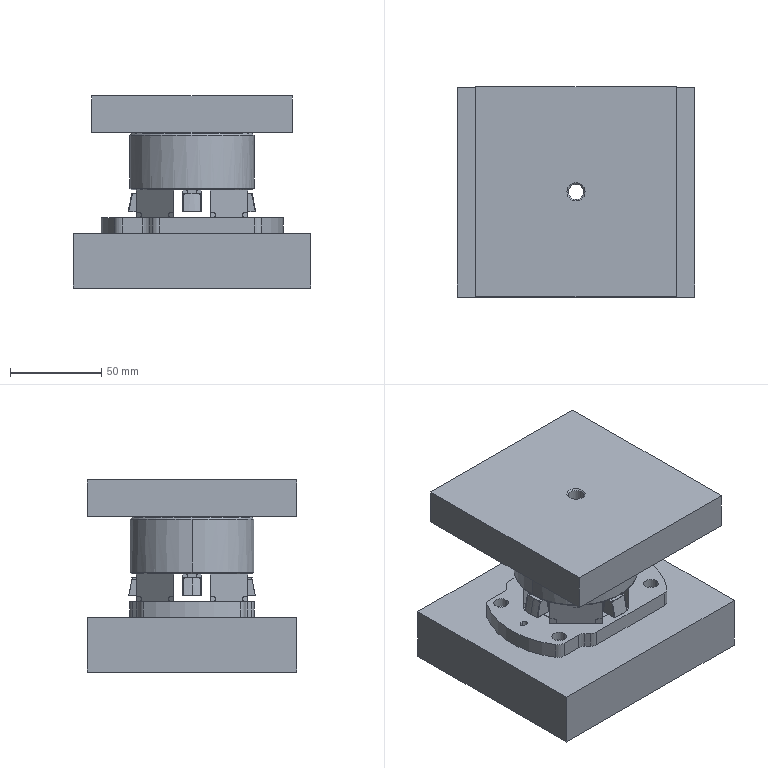NC program | NX | posted with a generic post | part box 130 x 115 x 105.2 mm
Lines 1 to 950 of 2949:
N10 G17 G21 G94 G90
(PLANAR_MILL_COPY_4_COPY_3_COPY_1 , TOOL : D2)
N12 T20 M6
N14 G54
N16 G17 G0 G90 X-1.137 Y30.713 S6000 M3
N18 G43 Z52.144 H20
N20 G94 G1 Y9.394 Z30.825 F5000.
N22 G41 X-1. Y9.659 Z30.559 F1200. D20
N24 Y11.721 Z28.498
N26 X-1.018 Y11.795 Z28.423
N28 X-1.095 Y11.849 Z28.369
N30 X-1.2 Y11.862 Z28.356
N32 X-1.8
N34 X-1.905 Y11.849 Z28.369
N36 X-1.982 Y11.795 Z28.423
N38 X-2. Y11.721 Z28.498
N40 Y9.894 Z30.324
N42 X-1.966 Y9.827 Z30.391
N44 G40
N46 X-1.863 Y9.628 Z30.59
N48 G0 X-1.137 Y9.288 Z30.719
N50 G41 G1 X-1. Y9.553 Z30.453
N52 Y11.615 Z28.392
N54 X-1.018 Y11.689 Z28.317
N56 X-1.095 Y11.743 Z28.263
N58 X-1.2 Y11.756 Z28.25
N60 X-1.8
N62 X-1.905 Y11.743 Z28.263
N64 X-1.982 Y11.689 Z28.317
N66 X-2. Y11.615 Z28.392
N68 Y9.788 Z30.218
N70 X-1.966 Y9.721 Z30.285
N72 G40
N74 X-1.863 Y9.522 Z30.484
N76 G0 X-1.137 Y9.182 Z30.613
N78 G41 G1 X-1. Y9.447 Z30.347
N80 Y11.509 Z28.286
N82 X-1.018 Y11.583 Z28.211
N84 X-1.095 Y11.637 Z28.157
N86 X-1.2 Y11.65 Z28.144
N88 X-1.8
N90 X-1.905 Y11.637 Z28.157
N92 X-1.982 Y11.583 Z28.211
N94 X-2. Y11.509 Z28.286
N96 Y9.682 Z30.112
N98 X-1.966 Y9.615 Z30.179
N100 G40
N102 X-1.863 Y9.416 Z30.378
N104 G0 X-1.137 Y9.076 Z30.507
N106 G41 G1 X-1. Y9.341 Z30.241
N108 Y11.403 Z28.179
N110 X-1.018 Y11.477 Z28.105
N112 X-1.095 Y11.531 Z28.051
N114 X-1.2 Y11.544 Z28.038
N116 X-1.8
N118 X-1.905 Y11.531 Z28.051
N120 X-1.982 Y11.477 Z28.105
N122 X-2. Y11.403 Z28.179
N124 Y9.576 Z30.006
N126 X-1.966 Y9.509 Z30.073
N128 G40
N130 X-1.863 Y9.31 Z30.272
N132 G0 X-1.137 Y8.969 Z30.4
N134 G41 G1 X-1. Y9.235 Z30.135
N136 Y11.296 Z28.073
N138 X-1.018 Y11.371 Z27.999
N140 X-1.095 Y11.425 Z27.945
N142 X-1.2 Y11.438 Z27.932
N144 X-1.8
N146 X-1.905 Y11.425 Z27.945
N148 X-1.982 Y11.371 Z27.999
N150 X-2. Y11.296 Z28.073
N152 Y9.47 Z29.9
N154 X-1.966 Y9.403 Z29.967
N156 G40
N158 X-1.863 Y9.204 Z30.166
N160 G0 X-1.137 Y8.863 Z30.294
N162 G41 G1 X-1. Y9.129 Z30.029
N164 Y11.19 Z27.967
N166 X-1.018 Y11.265 Z27.893
N168 X-1.095 Y11.319 Z27.839
N170 X-1.2 Y11.332 Z27.826
N172 X-1.8
N174 X-1.905 Y11.319 Z27.839
N176 X-1.982 Y11.265 Z27.893
N178 X-2. Y11.19 Z27.967
N180 Y9.364 Z29.794
N182 X-1.966 Y9.297 Z29.861
N184 G40
N186 X-1.863 Y9.098 Z30.06
N188 G0 X-1.137 Y8.757 Z30.188
N190 G41 G1 X-1. Y9.023 Z29.923
N192 Y11.084 Z27.861
N194 X-1.018 Y11.159 Z27.787
N196 X-1.095 Y11.213 Z27.733
N198 X-1.2 Y11.226 Z27.72
N200 X-1.8
N202 X-1.905 Y11.213 Z27.733
N204 X-1.982 Y11.159 Z27.787
N206 X-2. Y11.084 Z27.861
N208 Y9.258 Z29.688
N210 X-1.966 Y9.191 Z29.755
N212 G40
N214 X-1.863 Y8.992 Z29.954
N216 G0 X-1.137 Y8.651 Z30.082
N218 G41 G1 X-1. Y8.917 Z29.816
N220 Y10.978 Z27.755
N222 X-1.018 Y11.053 Z27.681
N224 X-1.095 Y11.107 Z27.627
N226 X-1.2 Y11.12 Z27.614
N228 X-1.8
N230 X-1.905 Y11.107 Z27.627
N232 X-1.982 Y11.053 Z27.681
N234 X-2. Y10.978 Z27.755
N236 Y9.151 Z29.582
N238 X-1.966 Y9.085 Z29.648
N240 G40
N242 X-1.863 Y8.886 Z29.848
N244 G0 X-1.137 Y8.545 Z29.976
N246 G41 G1 X-1. Y8.811 Z29.71
N248 Y10.872 Z27.649
N250 X-1.018 Y10.946 Z27.575
N252 X-1.095 Y11.001 Z27.521
N254 X-1.2 Y11.014 Z27.508
N256 X-1.8
N258 X-1.905 Y11.001 Z27.521
N260 X-1.982 Y10.946 Z27.575
N262 X-2. Y10.872 Z27.649
N264 Y9.045 Z29.476
N266 X-1.966 Y8.979 Z29.542
N268 G40
N270 X-1.863 Y8.78 Z29.742
N272 G0 X-1.137 Y8.439 Z29.87
N274 G41 G1 X-1. Y8.705 Z29.604
N276 Y10.766 Z27.543
N278 X-1.018 Y10.84 Z27.469
N280 X-1.095 Y10.895 Z27.414
N282 X-1.2 Y10.908 Z27.402
N284 X-1.8
N286 X-1.905 Y10.895 Z27.414
N288 X-1.982 Y10.84 Z27.469
N290 X-2. Y10.766 Z27.543
N292 Y8.939 Z29.37
N294 X-1.966 Y8.873 Z29.436
N296 G40
N298 X-1.863 Y8.674 Z29.636
N300 G0 X-1.137 Y8.333 Z29.764
N302 G41 G1 X-1. Y8.599 Z29.498
N304 Y10.66 Z27.437
N306 X-1.018 Y10.734 Z27.363
N308 X-1.095 Y10.789 Z27.308
N310 X-1.2 Y10.802 Z27.296
N312 X-1.8
N314 X-1.905 Y10.789 Z27.308
N316 X-1.982 Y10.734 Z27.363
N318 X-2. Y10.66 Z27.437
N320 Y8.833 Z29.264
N322 X-1.966 Y8.767 Z29.33
N324 G40
N326 X-1.863 Y8.567 Z29.53
N328 G0 X-1.137 Y8.227 Z29.658
N330 G41 G1 X-1. Y8.493 Z29.392
N332 Y10.554 Z27.331
N334 X-1.018 Y10.628 Z27.257
N336 X-1.095 Y10.683 Z27.202
N338 X-1.2 Y10.695 Z27.19
N340 X-1.8
N342 X-1.905 Y10.683 Z27.202
N344 X-1.982 Y10.628 Z27.257
N346 X-2. Y10.554 Z27.331
N348 Y8.727 Z29.158
N350 X-1.966 Y8.661 Z29.224
N352 G40
N354 X-1.863 Y8.461 Z29.424
N356 G0 X-1.137 Y8.121 Z29.552
N358 G41 G1 X-1. Y8.387 Z29.286
N360 Y10.448 Z27.225
N362 X-1.018 Y10.522 Z27.151
N364 X-1.095 Y10.577 Z27.096
N366 X-1.2 Y10.589 Z27.083
N368 X-1.8
N370 X-1.905 Y10.577 Z27.096
N372 X-1.982 Y10.522 Z27.151
N374 X-2. Y10.448 Z27.225
N376 Y8.621 Z29.052
N378 X-1.966 Y8.555 Z29.118
N380 G40
N382 X-1.863 Y8.355 Z29.317
N384 G0 X-1.137 Y8.015 Z29.446
N386 G41 G1 X-1. Y8.281 Z29.18
N388 Y10.342 Z27.119
N390 X-1.018 Y10.416 Z27.045
N392 X-1.095 Y10.47 Z26.99
N394 X-1.2 Y10.483 Z26.977
N396 X-1.8
N398 X-1.905 Y10.47 Z26.99
N400 X-1.982 Y10.416 Z27.045
N402 X-2. Y10.342 Z27.119
N404 Y8.515 Z28.946
N406 X-1.966 Y8.449 Z29.012
N408 G40
N410 X-1.863 Y8.249 Z29.211
N412 G0 X-1.137 Y7.909 Z29.34
N414 G41 G1 X-1. Y8.175 Z29.074
N416 Y10.236 Z27.013
N418 X-1.018 Y10.31 Z26.939
N420 X-1.095 Y10.364 Z26.884
N422 X-1.2 Y10.377 Z26.871
N424 X-1.8
N426 X-1.905 Y10.364 Z26.884
N428 X-1.982 Y10.31 Z26.939
N430 X-2. Y10.236 Z27.013
N432 Y8.409 Z28.84
N434 X-1.966 Y8.343 Z28.906
N436 G40
N438 X-1.863 Y8.143 Z29.105
N440 G0 X-1.137 Y7.803 Z29.234
N442 G41 G1 X-1. Y8.069 Z28.968
N444 Y10.13 Z26.907
N446 X-1.018 Y10.204 Z26.832
N448 X-1.095 Y10.258 Z26.778
N450 X-1.2 Y10.271 Z26.765
N452 X-1.8
N454 X-1.905 Y10.258 Z26.778
N456 X-1.982 Y10.204 Z26.832
N458 X-2. Y10.13 Z26.907
N460 Y8.303 Z28.734
N462 X-1.966 Y8.236 Z28.8
N464 G40
N466 X-1.863 Y8.037 Z28.999
N468 G0 X-1.137 Y7.697 Z29.128
N470 G41 G1 X-1. Y7.962 Z28.862
N472 Y10.024 Z26.801
N474 X-1.018 Y10.098 Z26.726
N476 X-1.095 Y10.152 Z26.672
N478 X-1.2 Y10.165 Z26.659
N480 X-1.8
N482 X-1.905 Y10.152 Z26.672
N484 X-1.982 Y10.098 Z26.726
N486 X-2. Y10.024 Z26.801
N488 Y8.197 Z28.627
N490 X-1.966 Y8.13 Z28.694
N492 G40
N494 X-1.863 Y7.931 Z28.893
N496 G0 X-1.137 Y7.591 Z29.022
N498 G41 G1 X-1. Y7.856 Z28.756
N500 Y9.918 Z26.695
N502 X-1.018 Y9.992 Z26.62
N504 X-1.095 Y10.046 Z26.566
N506 X-1.2 Y10.059 Z26.553
N508 X-1.8
N510 X-1.905 Y10.046 Z26.566
N512 X-1.982 Y9.992 Z26.62
N514 X-2. Y9.918 Z26.695
N516 Y8.091 Z28.521
N518 X-1.966 Y8.024 Z28.588
N520 G40
N522 X-1.863 Y7.825 Z28.787
N524 G0 X-1.137 Y7.485 Z28.916
N526 G41 G1 X-1. Y7.75 Z28.65
N528 Y9.812 Z26.588
N530 X-1.018 Y9.886 Z26.514
N532 X-1.095 Y9.94 Z26.46
N534 X-1.2 Y9.953 Z26.447
N536 X-1.8
N538 X-1.905 Y9.94 Z26.46
N540 X-1.982 Y9.886 Z26.514
N542 X-2. Y9.812 Z26.588
N544 Y7.985 Z28.415
N546 X-1.966 Y7.918 Z28.482
N548 G40
N550 X-1.863 Y7.719 Z28.681
N552 G0 X-1.137 Y7.378 Z28.809
N554 G41 G1 X-1. Y7.644 Z28.544
N556 Y9.705 Z26.482
N558 X-1.018 Y9.78 Z26.408
N560 X-1.095 Y9.834 Z26.354
N562 X-1.2 Y9.847 Z26.341
N564 X-1.8
N566 X-1.905 Y9.834 Z26.354
N568 X-1.982 Y9.78 Z26.408
N570 X-2. Y9.705 Z26.482
N572 Y7.879 Z28.309
N574 X-1.966 Y7.812 Z28.376
N576 G40
N578 X-1.863 Y7.613 Z28.575
N580 G0 X-1.137 Y7.272 Z28.703
N582 G41 G1 X-1. Y7.538 Z28.438
N584 Y9.599 Z26.376
N586 X-1.018 Y9.674 Z26.302
N588 X-1.095 Y9.728 Z26.248
N590 X-1.2 Y9.741 Z26.235
N592 X-1.8
N594 X-1.905 Y9.728 Z26.248
N596 X-1.982 Y9.674 Z26.302
N598 X-2. Y9.599 Z26.376
N600 Y7.773 Z28.203
N602 X-1.966 Y7.706 Z28.27
N604 G40
N606 X-1.863 Y7.507 Z28.469
N608 G0 X-1.137 Y7.166 Z28.597
N610 G41 G1 X-1. Y7.432 Z28.332
N612 Y9.493 Z26.27
N614 X-1.018 Y9.568 Z26.196
N616 X-1.095 Y9.622 Z26.142
N618 X-1.2 Y9.635 Z26.129
N620 X-1.8
N622 X-1.905 Y9.622 Z26.142
N624 X-1.982 Y9.568 Z26.196
N626 X-2. Y9.493 Z26.27
N628 Y7.667 Z28.097
N630 X-1.966 Y7.6 Z28.164
N632 G40
N634 X-1.863 Y7.401 Z28.363
N636 G0 X-1.137 Y7.06 Z28.491
N638 G41 G1 X-1. Y7.326 Z28.225
N640 Y9.387 Z26.164
N642 X-1.018 Y9.462 Z26.09
N644 X-1.095 Y9.516 Z26.036
N646 X-1.2 Y9.529 Z26.023
N648 X-1.8
N650 X-1.905 Y9.516 Z26.036
N652 X-1.982 Y9.462 Z26.09
N654 X-2. Y9.387 Z26.164
N656 Y7.56 Z27.991
N658 X-1.966 Y7.494 Z28.057
N660 G40
N662 X-1.863 Y7.295 Z28.257
N664 G0 X-1.137 Y6.954 Z28.385
N666 G41 G1 X-1. Y7.22 Z28.119
N668 Y9.281 Z26.058
N670 X-1.018 Y9.355 Z25.984
N672 X-1.095 Y9.41 Z25.93
N674 X-1.2 Y9.423 Z25.917
N676 X-1.8
N678 X-1.905 Y9.41 Z25.93
N680 X-1.982 Y9.355 Z25.984
N682 X-2. Y9.281 Z26.058
N684 Y7.454 Z27.885
N686 X-1.966 Y7.388 Z27.951
N688 G40
N690 X-1.863 Y7.189 Z28.151
N692 G0 X-1.137 Y6.848 Z28.279
N694 G41 G1 X-1. Y7.114 Z28.013
N696 Y9.175 Z25.952
N698 X-1.018 Y9.249 Z25.878
N700 X-1.095 Y9.304 Z25.824
N702 X-1.2 Y9.317 Z25.811
N704 X-1.8
N706 X-1.905 Y9.304 Z25.824
N708 X-1.982 Y9.249 Z25.878
N710 X-2. Y9.175 Z25.952
N712 Y7.348 Z27.779
N714 X-1.966 Y7.282 Z27.845
N716 G40
N718 X-1.863 Y7.083 Z28.045
N720 G0 X-1.137 Y6.813 Z28.244
N722 G41 G1 X-1. Y7.079 Z27.978
N724 Y9.14 Z25.917
N726 X-1.018 Y9.214 Z25.843
N728 X-1.095 Y9.268 Z25.788
N730 X-1.2 Y9.281 Z25.775
N732 X-1.8
N734 X-1.905 Y9.268 Z25.788
N736 X-1.982 Y9.214 Z25.843
N738 X-2. Y9.14 Z25.917
N740 Y7.313 Z27.744
N742 X-1.966 Y7.247 Z27.81
N744 G40
N746 X-1.863 Y7.047 Z28.009
N748 G0 Y27.412 Z48.374
N750 Y48.374 Z27.412
N752 G1 Y30.59 Z9.628 F5000.
N754 G41 X-2. Y30.324 Z9.894 F1200.
N756 Y28.498 Z11.721
N758 X-1.982 Y28.423 Z11.795
N760 X-1.905 Y28.369 Z11.849
N762 X-1.8 Y28.356 Z11.862
N764 X-1.2
N766 X-1.095 Y28.369 Z11.849
N768 X-1.018 Y28.423 Z11.795
N770 X-1. Y28.498 Z11.721
N772 Y30.559 Z9.659
N774 X-1.034 Y30.625 Z9.593
N776 G40
N778 X-1.137 Y30.825 Z9.394
N780 G0 X-1.863 Y30.484 Z9.522
N782 G41 G1 X-2. Y30.218 Z9.788
N784 Y28.392 Z11.615
N786 X-1.982 Y28.317 Z11.689
N788 X-1.905 Y28.263 Z11.743
N790 X-1.8 Y28.25 Z11.756
N792 X-1.2
N794 X-1.095 Y28.263 Z11.743
N796 X-1.018 Y28.317 Z11.689
N798 X-1. Y28.392 Z11.615
N800 Y30.453 Z9.553
N802 X-1.034 Y30.519 Z9.487
N804 G40
N806 X-1.137 Y30.719 Z9.288
N808 G0 X-1.863 Y30.378 Z9.416
N810 G41 G1 X-2. Y30.112 Z9.682
N812 Y28.286 Z11.509
N814 X-1.982 Y28.211 Z11.583
N816 X-1.905 Y28.157 Z11.637
N818 X-1.8 Y28.144 Z11.65
N820 X-1.2
N822 X-1.095 Y28.157 Z11.637
N824 X-1.018 Y28.211 Z11.583
N826 X-1. Y28.286 Z11.509
N828 Y30.347 Z9.447
N830 X-1.034 Y30.413 Z9.381
N832 G40
N834 X-1.137 Y30.613 Z9.182
N836 G0 X-1.863 Y30.272 Z9.31
N838 G41 G1 X-2. Y30.006 Z9.576
N840 Y28.179 Z11.403
N842 X-1.982 Y28.105 Z11.477
N844 X-1.905 Y28.051 Z11.531
N846 X-1.8 Y28.038 Z11.544
N848 X-1.2
N850 X-1.095 Y28.051 Z11.531
N852 X-1.018 Y28.105 Z11.477
N854 X-1. Y28.179 Z11.403
N856 Y30.241 Z9.341
N858 X-1.034 Y30.307 Z9.275
N860 G40
N862 X-1.137 Y30.507 Z9.076
N864 G0 X-1.863 Y30.166 Z9.204
N866 G41 G1 X-2. Y29.9 Z9.47
N868 Y28.073 Z11.296
N870 X-1.982 Y27.999 Z11.371
N872 X-1.905 Y27.945 Z11.425
N874 X-1.8 Y27.932 Z11.438
N876 X-1.2
N878 X-1.095 Y27.945 Z11.425
N880 X-1.018 Y27.999 Z11.371
N882 X-1. Y28.073 Z11.296
N884 Y30.135 Z9.235
N886 X-1.034 Y30.201 Z9.169
N888 G40
N890 X-1.137 Y30.4 Z8.969
N892 G0 X-1.863 Y30.06 Z9.098
N894 G41 G1 X-2. Y29.794 Z9.364
N896 Y27.967 Z11.19
N898 X-1.982 Y27.893 Z11.265
N900 X-1.905 Y27.839 Z11.319
N902 X-1.8 Y27.826 Z11.332
N904 X-1.2
N906 X-1.095 Y27.839 Z11.319
N908 X-1.018 Y27.893 Z11.265
N910 X-1. Y27.967 Z11.19
N912 Y30.029 Z9.129
N914 X-1.034 Y30.095 Z9.063
N916 G40
N918 X-1.137 Y30.294 Z8.863
N920 G0 X-1.863 Y29.954 Z8.992
N922 G41 G1 X-2. Y29.688 Z9.258
N924 Y27.861 Z11.084
N926 X-1.982 Y27.787 Z11.159
N928 X-1.905 Y27.733 Z11.213
N930 X-1.8 Y27.72 Z11.226
N932 X-1.2
N934 X-1.095 Y27.733 Z11.213
N936 X-1.018 Y27.787 Z11.159
N938 X-1. Y27.861 Z11.084
N940 Y29.923 Z9.023
N942 X-1.034 Y29.989 Z8.957
N944 G40
N946 X-1.137 Y30.188 Z8.757
N948 G0 X-1.863 Y29.848 Z8.886
N950 G41 G1 X-2. Y29.582 Z9.151
N952 Y27.755 Z10.978
N954 X-1.982 Y27.681 Z11.053
N956 X-1.905 Y27.627 Z11.107
N958 X-1.8 Y27.614 Z11.12
N960 X-1.2
N962 X-1.095 Y27.627 Z11.107
N964 X-1.018 Y27.681 Z11.053
N966 X-1. Y27.755 Z10.978
N968 Y29.816 Z8.917
N970 X-1.034 Y29.883 Z8.851
N972 G40
N974 X-1.137 Y30.082 Z8.651
N976 G0 X-1.863 Y29.742 Z8.78
N978 G41 G1 X-2. Y29.476 Z9.045
N980 Y27.649 Z10.872
N982 X-1.982 Y27.575 Z10.946
N984 X-1.905 Y27.521 Z11.001
N986 X-1.8 Y27.508 Z11.014
N988 X-1.2
N990 X-1.095 Y27.521 Z11.001
N992 X-1.018 Y27.575 Z10.946
N994 X-1. Y27.649 Z10.872
N996 Y29.71 Z8.811
N998 X-1.034 Y29.777 Z8.745
N1000 G40
N1002 X-1.137 Y29.976 Z8.545
N1004 G0 X-1.863 Y29.636 Z8.674
N1006 G41 G1 X-2. Y29.37 Z8.939
N1008 Y27.543 Z10.766
N1010 X-1.982 Y27.469 Z10.84
N1012 X-1.905 Y27.414 Z10.895
N1014 X-1.8 Y27.402 Z10.908
N1016 X-1.2
N1018 X-1.095 Y27.414 Z10.895
N1020 X-1.018 Y27.469 Z10.84
N1022 X-1. Y27.543 Z10.766
N1024 Y29.604 Z8.705
N1026 X-1.034 Y29.671 Z8.638
N1028 G40
N1030 X-1.137 Y29.87 Z8.439
N1032 G0 X-1.863 Y29.53 Z8.567
N1034 G41 G1 X-2. Y29.264 Z8.833
N1036 Y27.437 Z10.66
N1038 X-1.982 Y27.363 Z10.734
N1040 X-1.905 Y27.308 Z10.789
N1042 X-1.8 Y27.296 Z10.802
N1044 X-1.2
N1046 X-1.095 Y27.308 Z10.789
N1048 X-1.018 Y27.363 Z10.734
N1050 X-1. Y27.437 Z10.66
N1052 Y29.498 Z8.599
N1054 X-1.034 Y29.565 Z8.532
N1056 G40
N1058 X-1.137 Y29.764 Z8.333
N1060 G0 X-1.863 Y29.424 Z8.461
N1062 G41 G1 X-2. Y29.158 Z8.727
N1064 Y27.331 Z10.554
N1066 X-1.982 Y27.257 Z10.628
N1068 X-1.905 Y27.202 Z10.683
N1070 X-1.8 Y27.19 Z10.695
N1072 X-1.2
N1074 X-1.095 Y27.202 Z10.683
N1076 X-1.018 Y27.257 Z10.628
N1078 X-1. Y27.331 Z10.554
N1080 Y29.392 Z8.493
N1082 X-1.034 Y29.459 Z8.426
N1084 G40
N1086 X-1.137 Y29.658 Z8.227
N1088 G0 X-1.863 Y29.317 Z8.355
N1090 G41 G1 X-2. Y29.052 Z8.621
N1092 Y27.225 Z10.448
N1094 X-1.982 Y27.151 Z10.522
N1096 X-1.905 Y27.096 Z10.577
N1098 X-1.8 Y27.083 Z10.589
N1100 X-1.2
N1102 X-1.095 Y27.096 Z10.577
N1104 X-1.018 Y27.151 Z10.522
N1106 X-1. Y27.225 Z10.448
N1108 Y29.286 Z8.387
N1110 X-1.034 Y29.353 Z8.32
N1112 G40
N1114 X-1.137 Y29.552 Z8.121
N1116 G0 X-1.863 Y29.211 Z8.249
N1118 G41 G1 X-2. Y28.946 Z8.515
N1120 Y27.119 Z10.342
N1122 X-1.982 Y27.045 Z10.416
N1124 X-1.905 Y26.99 Z10.47
N1126 X-1.8 Y26.977 Z10.483
N1128 X-1.2
N1130 X-1.095 Y26.99 Z10.47
N1132 X-1.018 Y27.045 Z10.416
N1134 X-1. Y27.119 Z10.342
N1136 Y29.18 Z8.281
N1138 X-1.034 Y29.247 Z8.214
N1140 G40
N1142 X-1.137 Y29.446 Z8.015
N1144 G0 X-1.863 Y29.105 Z8.143
N1146 G41 G1 X-2. Y28.84 Z8.409
N1148 Y27.013 Z10.236
N1150 X-1.982 Y26.939 Z10.31
N1152 X-1.905 Y26.884 Z10.364
N1154 X-1.8 Y26.871 Z10.377
N1156 X-1.2
N1158 X-1.095 Y26.884 Z10.364
N1160 X-1.018 Y26.939 Z10.31
N1162 X-1. Y27.013 Z10.236
N1164 Y29.074 Z8.175
N1166 X-1.034 Y29.14 Z8.108
N1168 G40
N1170 X-1.137 Y29.34 Z7.909
N1172 G0 X-1.863 Y28.999 Z8.037
N1174 G41 G1 X-2. Y28.734 Z8.303
N1176 Y26.907 Z10.13
N1178 X-1.982 Y26.832 Z10.204
N1180 X-1.905 Y26.778 Z10.258
N1182 X-1.8 Y26.765 Z10.271
N1184 X-1.2
N1186 X-1.095 Y26.778 Z10.258
N1188 X-1.018 Y26.832 Z10.204
N1190 X-1. Y26.907 Z10.13
N1192 Y28.968 Z8.069
N1194 X-1.034 Y29.034 Z8.002
N1196 G40
N1198 X-1.137 Y29.234 Z7.803
N1200 G0 X-1.863 Y28.893 Z7.931
N1202 G41 G1 X-2. Y28.627 Z8.197
N1204 Y26.801 Z10.024
N1206 X-1.982 Y26.726 Z10.098
N1208 X-1.905 Y26.672 Z10.152
N1210 X-1.8 Y26.659 Z10.165
N1212 X-1.2
N1214 X-1.095 Y26.672 Z10.152
N1216 X-1.018 Y26.726 Z10.098
N1218 X-1. Y26.801 Z10.024
N1220 Y28.862 Z7.962
N1222 X-1.034 Y28.928 Z7.896
N1224 G40
N1226 X-1.137 Y29.128 Z7.697
N1228 G0 X-1.863 Y28.787 Z7.825
N1230 G41 G1 X-2. Y28.521 Z8.091
N1232 Y26.695 Z9.918
N1234 X-1.982 Y26.62 Z9.992
N1236 X-1.905 Y26.566 Z10.046
N1238 X-1.8 Y26.553 Z10.059
N1240 X-1.2
N1242 X-1.095 Y26.566 Z10.046
N1244 X-1.018 Y26.62 Z9.992
N1246 X-1. Y26.695 Z9.918
N1248 Y28.756 Z7.856
N1250 X-1.034 Y28.822 Z7.79
N1252 G40
N1254 X-1.137 Y29.022 Z7.591
N1256 G0 X-1.863 Y28.681 Z7.719
N1258 G41 G1 X-2. Y28.415 Z7.985
N1260 Y26.588 Z9.812
N1262 X-1.982 Y26.514 Z9.886
N1264 X-1.905 Y26.46 Z9.94
N1266 X-1.8 Y26.447 Z9.953
N1268 X-1.2
N1270 X-1.095 Y26.46 Z9.94
N1272 X-1.018 Y26.514 Z9.886
N1274 X-1. Y26.588 Z9.812
N1276 Y28.65 Z7.75
N1278 X-1.034 Y28.716 Z7.684
N1280 G40
N1282 X-1.137 Y28.916 Z7.485
N1284 G0 X-1.863 Y28.575 Z7.613
N1286 G41 G1 X-2. Y28.309 Z7.879
N1288 Y26.482 Z9.705
N1290 X-1.982 Y26.408 Z9.78
N1292 X-1.905 Y26.354 Z9.834
N1294 X-1.8 Y26.341 Z9.847
N1296 X-1.2
N1298 X-1.095 Y26.354 Z9.834
N1300 X-1.018 Y26.408 Z9.78
N1302 X-1. Y26.482 Z9.705
N1304 Y28.544 Z7.644
N1306 X-1.034 Y28.61 Z7.578
N1308 G40
N1310 X-1.137 Y28.809 Z7.378
N1312 G0 X-1.863 Y28.469 Z7.507
N1314 G41 G1 X-2. Y28.203 Z7.773
N1316 Y26.376 Z9.599
N1318 X-1.982 Y26.302 Z9.674
N1320 X-1.905 Y26.248 Z9.728
N1322 X-1.8 Y26.235 Z9.741
N1324 X-1.2
N1326 X-1.095 Y26.248 Z9.728
N1328 X-1.018 Y26.302 Z9.674
N1330 X-1. Y26.376 Z9.599
N1332 Y28.438 Z7.538
N1334 X-1.034 Y28.504 Z7.472
N1336 G40
N1338 X-1.137 Y28.703 Z7.272
N1340 G0 X-1.863 Y28.363 Z7.401
N1342 G41 G1 X-2. Y28.097 Z7.667
N1344 Y26.27 Z9.493
N1346 X-1.982 Y26.196 Z9.568
N1348 X-1.905 Y26.142 Z9.622
N1350 X-1.8 Y26.129 Z9.635
N1352 X-1.2
N1354 X-1.095 Y26.142 Z9.622
N1356 X-1.018 Y26.196 Z9.568
N1358 X-1. Y26.27 Z9.493
N1360 Y28.332 Z7.432
N1362 X-1.034 Y28.398 Z7.366
N1364 G40
N1366 X-1.137 Y28.597 Z7.166
N1368 G0 X-1.863 Y28.257 Z7.295
N1370 G41 G1 X-2. Y27.991 Z7.56
N1372 Y26.164 Z9.387
N1374 X-1.982 Y26.09 Z9.462
N1376 X-1.905 Y26.036 Z9.516
N1378 X-1.8 Y26.023 Z9.529
N1380 X-1.2
N1382 X-1.095 Y26.036 Z9.516
N1384 X-1.018 Y26.09 Z9.462
N1386 X-1. Y26.164 Z9.387
N1388 Y28.225 Z7.326
N1390 X-1.034 Y28.292 Z7.26
N1392 G40
N1394 X-1.137 Y28.491 Z7.06
N1396 G0 X-1.863 Y28.151 Z7.189
N1398 G41 G1 X-2. Y27.885 Z7.454
N1400 Y26.058 Z9.281
N1402 X-1.982 Y25.984 Z9.355
N1404 X-1.905 Y25.93 Z9.41
N1406 X-1.8 Y25.917 Z9.423
N1408 X-1.2
N1410 X-1.095 Y25.93 Z9.41
N1412 X-1.018 Y25.984 Z9.355
N1414 X-1. Y26.058 Z9.281
N1416 Y28.119 Z7.22
N1418 X-1.034 Y28.186 Z7.154
N1420 G40
N1422 X-1.137 Y28.385 Z6.954
N1424 G0 X-1.863 Y28.045 Z7.083
N1426 G41 G1 X-2. Y27.779 Z7.348
N1428 Y25.952 Z9.175
N1430 X-1.982 Y25.878 Z9.249
N1432 X-1.905 Y25.824 Z9.304
N1434 X-1.8 Y25.811 Z9.317
N1436 X-1.2
N1438 X-1.095 Y25.824 Z9.304
N1440 X-1.018 Y25.878 Z9.249
N1442 X-1. Y25.952 Z9.175
N1444 Y28.013 Z7.114
N1446 X-1.034 Y28.08 Z7.047
N1448 G40
N1450 X-1.137 Y28.279 Z6.848
N1452 G0 X-1.863 Y28.009 Z7.047
N1454 G41 G1 X-2. Y27.744 Z7.313
N1456 Y25.917 Z9.14
N1458 X-1.982 Y25.843 Z9.214
N1460 X-1.905 Y25.788 Z9.268
N1462 X-1.8 Y25.775 Z9.281
N1464 X-1.2
N1466 X-1.095 Y25.788 Z9.268
N1468 X-1.018 Y25.843 Z9.214
N1470 X-1. Y25.917 Z9.14
N1472 Y27.978 Z7.079
N1474 X-1.034 Y28.044 Z7.012
N1476 G40
N1478 X-1.137 Y28.244 Z6.813
N1480 G0 Y52.144 Z30.713
(PLANAR_MILL_COPY_4_COPY_3_COPY_1_COPY , TOOL : D2)
N1482 Y-52.144
N1484 G1 Y-30.825 Z9.394 F5000.
N1486 G41 X-1. Y-30.559 Z9.659 F1200.
N1488 Y-28.498 Z11.721
N1490 X-1.018 Y-28.423 Z11.795
N1492 X-1.095 Y-28.369 Z11.849
N1494 X-1.2 Y-28.356 Z11.862
N1496 X-1.8
N1498 X-1.905 Y-28.369 Z11.849
N1500 X-1.982 Y-28.423 Z11.795
N1502 X-2. Y-28.498 Z11.721
N1504 Y-30.324 Z9.894
N1506 X-1.966 Y-30.391 Z9.827
N1508 G40
N1510 X-1.863 Y-30.59 Z9.628
N1512 G0 X-1.137 Y-30.719 Z9.288
N1514 G41 G1 X-1. Y-30.453 Z9.553
N1516 Y-28.392 Z11.615
N1518 X-1.018 Y-28.317 Z11.689
N1520 X-1.095 Y-28.263 Z11.743
N1522 X-1.2 Y-28.25 Z11.756
N1524 X-1.8
N1526 X-1.905 Y-28.263 Z11.743
N1528 X-1.982 Y-28.317 Z11.689
N1530 X-2. Y-28.392 Z11.615
N1532 Y-30.218 Z9.788
N1534 X-1.966 Y-30.285 Z9.721
N1536 G40
N1538 X-1.863 Y-30.484 Z9.522
N1540 G0 X-1.137 Y-30.613 Z9.182
N1542 G41 G1 X-1. Y-30.347 Z9.447
N1544 Y-28.286 Z11.509
N1546 X-1.018 Y-28.211 Z11.583
N1548 X-1.095 Y-28.157 Z11.637
N1550 X-1.2 Y-28.144 Z11.65
N1552 X-1.8
N1554 X-1.905 Y-28.157 Z11.637
N1556 X-1.982 Y-28.211 Z11.583
N1558 X-2. Y-28.286 Z11.509
N1560 Y-30.112 Z9.682
N1562 X-1.966 Y-30.179 Z9.615
N1564 G40
N1566 X-1.863 Y-30.378 Z9.416
N1568 G0 X-1.137 Y-30.507 Z9.076
N1570 G41 G1 X-1. Y-30.241 Z9.341
N1572 Y-28.179 Z11.403
N1574 X-1.018 Y-28.105 Z11.477
N1576 X-1.095 Y-28.051 Z11.531
N1578 X-1.2 Y-28.038 Z11.544
N1580 X-1.8
N1582 X-1.905 Y-28.051 Z11.531
N1584 X-1.982 Y-28.105 Z11.477
N1586 X-2. Y-28.179 Z11.403
N1588 Y-30.006 Z9.576
N1590 X-1.966 Y-30.073 Z9.509
N1592 G40
N1594 X-1.863 Y-30.272 Z9.31
N1596 G0 X-1.137 Y-30.4 Z8.969
N1598 G41 G1 X-1. Y-30.135 Z9.235
N1600 Y-28.073 Z11.296
N1602 X-1.018 Y-27.999 Z11.371
N1604 X-1.095 Y-27.945 Z11.425
N1606 X-1.2 Y-27.932 Z11.438
N1608 X-1.8
N1610 X-1.905 Y-27.945 Z11.425
N1612 X-1.982 Y-27.999 Z11.371
N1614 X-2. Y-28.073 Z11.296
N1616 Y-29.9 Z9.47
N1618 X-1.966 Y-29.967 Z9.403
N1620 G40
N1622 X-1.863 Y-30.166 Z9.204
N1624 G0 X-1.137 Y-30.294 Z8.863
N1626 G41 G1 X-1. Y-30.029 Z9.129
N1628 Y-27.967 Z11.19
N1630 X-1.018 Y-27.893 Z11.265
N1632 X-1.095 Y-27.839 Z11.319
N1634 X-1.2 Y-27.826 Z11.332
N1636 X-1.8
N1638 X-1.905 Y-27.839 Z11.319
N1640 X-1.982 Y-27.893 Z11.265
N1642 X-2. Y-27.967 Z11.19
N1644 Y-29.794 Z9.364
N1646 X-1.966 Y-29.861 Z9.297
N1648 G40
N1650 X-1.863 Y-30.06 Z9.098
N1652 G0 X-1.137 Y-30.188 Z8.757
N1654 G41 G1 X-1. Y-29.923 Z9.023
N1656 Y-27.861 Z11.084
N1658 X-1.018 Y-27.787 Z11.159
N1660 X-1.095 Y-27.733 Z11.213
N1662 X-1.2 Y-27.72 Z11.226
N1664 X-1.8
N1666 X-1.905 Y-27.733 Z11.213
N1668 X-1.982 Y-27.787 Z11.159
N1670 X-2. Y-27.861 Z11.084
N1672 Y-29.688 Z9.258
N1674 X-1.966 Y-29.755 Z9.191
N1676 G40
N1678 X-1.863 Y-29.954 Z8.992
N1680 G0 X-1.137 Y-30.082 Z8.651
N1682 G41 G1 X-1. Y-29.816 Z8.917
N1684 Y-27.755 Z10.978
N1686 X-1.018 Y-27.681 Z11.053
N1688 X-1.095 Y-27.627 Z11.107
N1690 X-1.2 Y-27.614 Z11.12
N1692 X-1.8
N1694 X-1.905 Y-27.627 Z11.107
N1696 X-1.982 Y-27.681 Z11.053
N1698 X-2. Y-27.755 Z10.978
N1700 Y-29.582 Z9.151
N1702 X-1.966 Y-29.648 Z9.085
N1704 G40
N1706 X-1.863 Y-29.848 Z8.886
N1708 G0 X-1.137 Y-29.976 Z8.545
N1710 G41 G1 X-1. Y-29.71 Z8.811
N1712 Y-27.649 Z10.872
N1714 X-1.018 Y-27.575 Z10.946
N1716 X-1.095 Y-27.521 Z11.001
N1718 X-1.2 Y-27.508 Z11.014
N1720 X-1.8
N1722 X-1.905 Y-27.521 Z11.001
N1724 X-1.982 Y-27.575 Z10.946
N1726 X-2. Y-27.649 Z10.872
N1728 Y-29.476 Z9.045
N1730 X-1.966 Y-29.542 Z8.979
N1732 G40
N1734 X-1.863 Y-29.742 Z8.78
N1736 G0 X-1.137 Y-29.87 Z8.439
N1738 G41 G1 X-1. Y-29.604 Z8.705
N1740 Y-27.543 Z10.766
N1742 X-1.018 Y-27.469 Z10.84
N1744 X-1.095 Y-27.414 Z10.895
N1746 X-1.2 Y-27.402 Z10.908
N1748 X-1.8
N1750 X-1.905 Y-27.414 Z10.895
N1752 X-1.982 Y-27.469 Z10.84
N1754 X-2. Y-27.543 Z10.766
N1756 Y-29.37 Z8.939
N1758 X-1.966 Y-29.436 Z8.873
N1760 G40
N1762 X-1.863 Y-29.636 Z8.674
N1764 G0 X-1.137 Y-29.764 Z8.333
N1766 G41 G1 X-1. Y-29.498 Z8.599
N1768 Y-27.437 Z10.66
N1770 X-1.018 Y-27.363 Z10.734
N1772 X-1.095 Y-27.308 Z10.789
N1774 X-1.2 Y-27.296 Z10.802
N1776 X-1.8
N1778 X-1.905 Y-27.308 Z10.789
N1780 X-1.982 Y-27.363 Z10.734
N1782 X-2. Y-27.437 Z10.66
N1784 Y-29.264 Z8.833
N1786 X-1.966 Y-29.33 Z8.767
N1788 G40
N1790 X-1.863 Y-29.53 Z8.567
N1792 G0 X-1.137 Y-29.658 Z8.227
N1794 G41 G1 X-1. Y-29.392 Z8.493
N1796 Y-27.331 Z10.554
N1798 X-1.018 Y-27.257 Z10.628
N1800 X-1.095 Y-27.202 Z10.683
N1802 X-1.2 Y-27.19 Z10.695
N1804 X-1.8
N1806 X-1.905 Y-27.202 Z10.683
N1808 X-1.982 Y-27.257 Z10.628
N1810 X-2. Y-27.331 Z10.554
N1812 Y-29.158 Z8.727
N1814 X-1.966 Y-29.224 Z8.661
N1816 G40
N1818 X-1.863 Y-29.424 Z8.461
N1820 G0 X-1.137 Y-29.552 Z8.121
N1822 G41 G1 X-1. Y-29.286 Z8.387
N1824 Y-27.225 Z10.448
N1826 X-1.018 Y-27.151 Z10.522
N1828 X-1.095 Y-27.096 Z10.577
N1830 X-1.2 Y-27.083 Z10.589
N1832 X-1.8
N1834 X-1.905 Y-27.096 Z10.577
N1836 X-1.982 Y-27.151 Z10.522
N1838 X-2. Y-27.225 Z10.448
N1840 Y-29.052 Z8.621
N1842 X-1.966 Y-29.118 Z8.555
N1844 G40
N1846 X-1.863 Y-29.317 Z8.355
N1848 G0 X-1.137 Y-29.446 Z8.015
N1850 G41 G1 X-1. Y-29.18 Z8.281
N1852 Y-27.119 Z10.342
N1854 X-1.018 Y-27.045 Z10.416
N1856 X-1.095 Y-26.99 Z10.47
N1858 X-1.2 Y-26.977 Z10.483
N1860 X-1.8
N1862 X-1.905 Y-26.99 Z10.47
N1864 X-1.982 Y-27.045 Z10.416
N1866 X-2. Y-27.119 Z10.342
N1868 Y-28.946 Z8.515
N1870 X-1.966 Y-29.012 Z8.449
N1872 G40
N1874 X-1.863 Y-29.211 Z8.249
N1876 G0 X-1.137 Y-29.34 Z7.909
N1878 G41 G1 X-1. Y-29.074 Z8.175
N1880 Y-27.013 Z10.236
N1882 X-1.018 Y-26.939 Z10.31
N1884 X-1.095 Y-26.884 Z10.364
N1886 X-1.2 Y-26.871 Z10.377
N1888 X-1.8
N1890 X-1.905 Y-26.884 Z10.364
N1892 X-1.982 Y-26.939 Z10.31